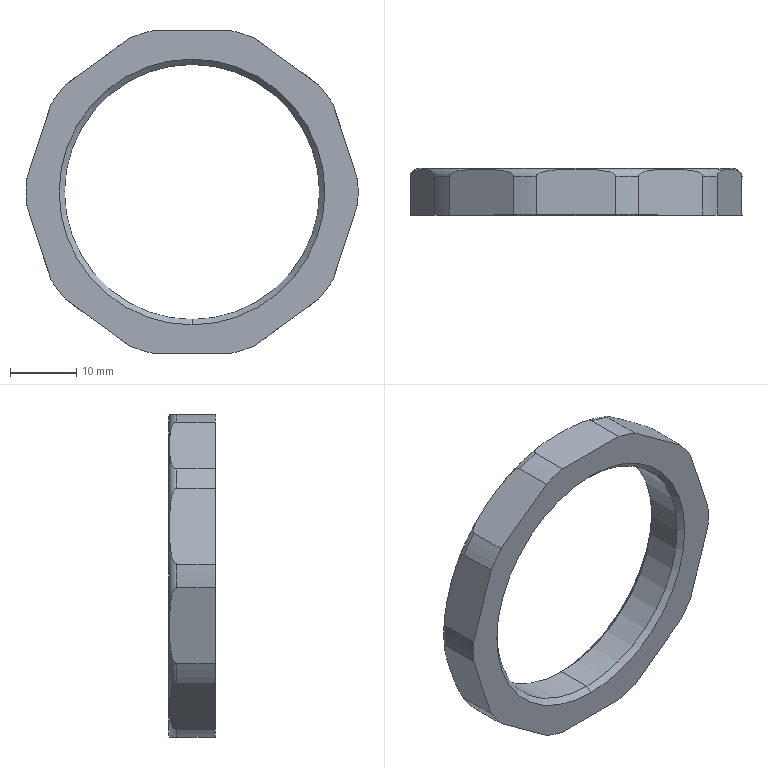Part | SolidWorks | features BaseBody 1 | 1 solid | 30 faces | box 50 x 7 x 48.544 mm | volume 5139 mm3 | cylinder 12 | plane 12 | cone 4 | torus 2 | commonest cylinder face diameters 50 x10 38.376 x2
STEP:
#1=CARTESIAN_POINT('',(5.99,38.8,-24.272));
#2=VERTEX_POINT('',#1);
#3=CARTESIAN_POINT('',(0.,39.903,-24.272));
#4=VERTEX_POINT('',#3);
#5=CARTESIAN_POINT('',(5.99,38.8,-24.272));
#6=CARTESIAN_POINT('',(5.99,38.868,-24.272));
#7=CARTESIAN_POINT('',(5.965,38.932,-24.272));
#8=CARTESIAN_POINT('',(5.891,39.043,-24.272));
#9=CARTESIAN_POINT('',(5.843,39.09,-24.272));
#10=CARTESIAN_POINT('',(5.688,39.215,-24.272));
#11=CARTESIAN_POINT('',(5.569,39.278,-24.272));
#12=CARTESIAN_POINT('',(5.208,39.438,-24.272));
#13=CARTESIAN_POINT('',(4.952,39.51,-24.272));
#14=CARTESIAN_POINT('',(4.439,39.627,-24.272));
#15=CARTESIAN_POINT('',(4.181,39.67,-24.272));
#16=CARTESIAN_POINT('',(3.663,39.742,-24.272));
#17=CARTESIAN_POINT('',(3.403,39.77,-24.272));
#18=CARTESIAN_POINT('',(2.621,39.838,-24.272));
#19=CARTESIAN_POINT('',(2.098,39.864,-24.272));
#20=CARTESIAN_POINT('',(1.049,39.897,-24.272));
#21=CARTESIAN_POINT('',(0.5246,39.903,-24.272));
#22=CARTESIAN_POINT('',(0.,39.903,-24.272));
#23=B_SPLINE_CURVE_WITH_KNOTS('',3,(#5,#6,#7,#8,#9,#10,#11,#12,#13,#14,#15,#16,#17,#18,#19,#20,#21,#22),.UNSPECIFIED.,.F.,.F.,(4,2,2,2,2,2,2,2,4),(-0.006293,-0.006096,-0.0059,-0.005506,-0.00472,-0.003933,-0.003146,-0.001573,0.),.UNSPECIFIED.);
#24=EDGE_CURVE('',#2,#4,#23,.T.);
#25=ORIENTED_EDGE('',*,*,#24,.T.);
#26=CARTESIAN_POINT('',(0.,40.,-23.8));
#27=VERTEX_POINT('',#26);
#28=CARTESIAN_POINT('',(0.,38.8,-23.8));
#29=DIRECTION('',(1.,0.,0.));
#30=DIRECTION('',(0.,0.,-1.));
#31=AXIS2_PLACEMENT_3D('',#28,#29,#30);
#32=CIRCLE('',#31,1.2);
#33=EDGE_CURVE('',#4,#27,#32,.T.);
#34=ORIENTED_EDGE('',*,*,#33,.T.);
#35=CARTESIAN_POINT('',(0.,40.,23.8));
#36=VERTEX_POINT('',#35);
#37=CARTESIAN_POINT('',(0.,40.,0.));
#38=DIRECTION('',(0.,-1.,0.));
#39=DIRECTION('',(0.,0.,1.));
#40=AXIS2_PLACEMENT_3D('',#37,#38,#39);
#41=CIRCLE('',#40,23.8);
#42=EDGE_CURVE('',#27,#36,#41,.T.);
#43=ORIENTED_EDGE('',*,*,#42,.T.);
#44=CARTESIAN_POINT('',(0.,39.903,24.272));
#45=VERTEX_POINT('',#44);
#46=CARTESIAN_POINT('',(0.,38.8,23.8));
#47=DIRECTION('',(-1.,0.,0.));
#48=DIRECTION('',(0.,0.,1.));
#49=AXIS2_PLACEMENT_3D('',#46,#47,#48);
#50=CIRCLE('',#49,1.2);
#51=EDGE_CURVE('',#45,#36,#50,.T.);
#52=ORIENTED_EDGE('',*,*,#51,.F.);
#53=CARTESIAN_POINT('',(5.99,38.8,24.272));
#54=VERTEX_POINT('',#53);
#55=CARTESIAN_POINT('',(0.,39.903,24.272));
#56=CARTESIAN_POINT('',(0.5253,39.903,24.272));
#57=CARTESIAN_POINT('',(1.05,39.897,24.272));
#58=CARTESIAN_POINT('',(2.1,39.864,24.272));
#59=CARTESIAN_POINT('',(2.625,39.838,24.272));
#60=CARTESIAN_POINT('',(3.672,39.746,24.272));
#61=CARTESIAN_POINT('',(4.195,39.683,24.272));
#62=CARTESIAN_POINT('',(4.963,39.507,24.272));
#63=CARTESIAN_POINT('',(5.218,39.435,24.272));
#64=CARTESIAN_POINT('',(5.577,39.274,24.272));
#65=CARTESIAN_POINT('',(5.693,39.212,24.272));
#66=CARTESIAN_POINT('',(5.846,39.087,24.272));
#67=CARTESIAN_POINT('',(5.894,39.04,24.272));
#68=CARTESIAN_POINT('',(5.965,38.931,24.272));
#69=CARTESIAN_POINT('',(5.99,38.867,24.272));
#70=CARTESIAN_POINT('',(5.99,38.8,24.272));
#71=B_SPLINE_CURVE_WITH_KNOTS('',3,(#55,#56,#57,#58,#59,#60,#61,#62,#63,#64,#65,#66,#67,#68,#69,#70),.UNSPECIFIED.,.F.,.F.,(4,2,2,2,2,2,2,4),(0.006368,0.007963,0.009557,0.01115,0.01195,0.01235,0.01255,0.01275),.UNSPECIFIED.);
#72=EDGE_CURVE('',#45,#54,#71,.T.);
#73=ORIENTED_EDGE('',*,*,#72,.T.);
#74=CARTESIAN_POINT('',(9.421,38.8,23.157));
#75=VERTEX_POINT('',#74);
#76=CARTESIAN_POINT('',(0.,38.8,0.));
#77=DIRECTION('',(0.,-1.,0.));
#78=DIRECTION('',(0.,0.,-1.));
#79=AXIS2_PLACEMENT_3D('',#76,#77,#78);
#80=CIRCLE('',#79,25.);
#81=EDGE_CURVE('',#75,#54,#80,.T.);
#82=ORIENTED_EDGE('',*,*,#81,.F.);
#83=CARTESIAN_POINT('',(19.112,38.8,16.116));
#84=VERTEX_POINT('',#83);
#85=CARTESIAN_POINT('',(9.421,38.8,23.157));
#86=CARTESIAN_POINT('',(9.421,38.868,23.157));
#87=CARTESIAN_POINT('',(9.441,38.932,23.142));
#88=CARTESIAN_POINT('',(9.501,39.043,23.099));
#89=CARTESIAN_POINT('',(9.54,39.091,23.071));
#90=CARTESIAN_POINT('',(9.665,39.215,22.979));
#91=CARTESIAN_POINT('',(9.762,39.278,22.909));
#92=CARTESIAN_POINT('',(10.054,39.438,22.697));
#93=CARTESIAN_POINT('',(10.261,39.51,22.546));
#94=CARTESIAN_POINT('',(10.676,39.627,22.245));
#95=CARTESIAN_POINT('',(10.885,39.671,22.093));
#96=CARTESIAN_POINT('',(11.305,39.742,21.788));
#97=CARTESIAN_POINT('',(11.515,39.77,21.635));
#98=CARTESIAN_POINT('',(12.148,39.838,21.175));
#99=CARTESIAN_POINT('',(12.572,39.864,20.867));
#100=CARTESIAN_POINT('',(13.421,39.897,20.251));
#101=CARTESIAN_POINT('',(13.846,39.903,19.942));
#102=CARTESIAN_POINT('',(14.695,39.903,19.325));
#103=CARTESIAN_POINT('',(15.12,39.896,19.017));
#104=CARTESIAN_POINT('',(15.968,39.863,18.4));
#105=CARTESIAN_POINT('',(16.393,39.838,18.092));
#106=CARTESIAN_POINT('',(17.239,39.746,17.477));
#107=CARTESIAN_POINT('',(17.662,39.683,17.17));
#108=CARTESIAN_POINT('',(18.282,39.507,16.719));
#109=CARTESIAN_POINT('',(18.488,39.435,16.569));
#110=CARTESIAN_POINT('',(18.779,39.274,16.358));
#111=CARTESIAN_POINT('',(18.873,39.212,16.29));
#112=CARTESIAN_POINT('',(18.997,39.087,16.2));
#113=CARTESIAN_POINT('',(19.035,39.04,16.172));
#114=CARTESIAN_POINT('',(19.093,38.931,16.13));
#115=CARTESIAN_POINT('',(19.112,38.867,16.116));
#116=CARTESIAN_POINT('',(19.112,38.8,16.116));
#117=B_SPLINE_CURVE_WITH_KNOTS('',3,(#85,#86,#87,#88,#89,#90,#91,#92,#93,#94,#95,#96,#97,#98,#99,#100,#101,#102,#103,#104,#105,#106,#107,#108,#109,#110,#111,#112,#113,#114,#115,#116),.UNSPECIFIED.,.F.,.F.,(4,2,2,2,2,2,2,2,2,2,2,2,2,2,2,4),(0.,0.0001992,0.0003983,0.0007966,0.001593,0.00239,0.003187,0.00478,0.006373,0.007966,0.00956,0.01115,0.01195,0.01235,0.01255,0.01275),.UNSPECIFIED.);
#118=EDGE_CURVE('',#75,#84,#117,.T.);
#119=ORIENTED_EDGE('',*,*,#118,.T.);
#120=CARTESIAN_POINT('',(21.233,38.8,13.197));
#121=VERTEX_POINT('',#120);
#122=CARTESIAN_POINT('',(0.,38.8,0.));
#123=DIRECTION('',(0.,-1.,0.));
#124=DIRECTION('',(0.,0.,-1.));
#125=AXIS2_PLACEMENT_3D('',#122,#123,#124);
#126=CIRCLE('',#125,25.);
#127=EDGE_CURVE('',#121,#84,#126,.T.);
#128=ORIENTED_EDGE('',*,*,#127,.F.);
#129=CARTESIAN_POINT('',(24.935,38.8,1.804));
#130=VERTEX_POINT('',#129);
#131=CARTESIAN_POINT('',(21.233,38.8,13.197));
#132=CARTESIAN_POINT('',(21.233,38.868,13.197));
#133=CARTESIAN_POINT('',(21.241,38.932,13.173));
#134=CARTESIAN_POINT('',(21.263,39.043,13.103));
#135=CARTESIAN_POINT('',(21.278,39.091,13.057));
#136=CARTESIAN_POINT('',(21.326,39.215,12.91));
#137=CARTESIAN_POINT('',(21.363,39.278,12.796));
#138=CARTESIAN_POINT('',(21.475,39.438,12.453));
#139=CARTESIAN_POINT('',(21.554,39.51,12.209));
#140=CARTESIAN_POINT('',(21.713,39.627,11.721));
#141=CARTESIAN_POINT('',(21.792,39.671,11.475));
#142=CARTESIAN_POINT('',(21.953,39.742,10.982));
#143=CARTESIAN_POINT('',(22.033,39.77,10.735));
#144=CARTESIAN_POINT('',(22.275,39.838,9.991));
#145=CARTESIAN_POINT('',(22.437,39.864,9.492));
#146=CARTESIAN_POINT('',(22.761,39.897,8.494));
#147=CARTESIAN_POINT('',(22.923,39.903,7.995));
#148=CARTESIAN_POINT('',(23.247,39.903,6.997));
#149=CARTESIAN_POINT('',(23.41,39.896,6.498));
#150=CARTESIAN_POINT('',(23.734,39.863,5.5));
#151=CARTESIAN_POINT('',(23.896,39.838,5.001));
#152=CARTESIAN_POINT('',(24.219,39.746,4.007));
#153=CARTESIAN_POINT('',(24.381,39.683,3.509));
#154=CARTESIAN_POINT('',(24.618,39.507,2.78));
#155=CARTESIAN_POINT('',(24.696,39.435,2.537));
#156=CARTESIAN_POINT('',(24.807,39.274,2.196));
#157=CARTESIAN_POINT('',(24.843,39.212,2.085));
#158=CARTESIAN_POINT('',(24.891,39.087,1.94));
#159=CARTESIAN_POINT('',(24.905,39.04,1.895));
#160=CARTESIAN_POINT('',(24.927,38.931,1.827));
#161=CARTESIAN_POINT('',(24.935,38.867,1.804));
#162=CARTESIAN_POINT('',(24.935,38.8,1.804));
#163=B_SPLINE_CURVE_WITH_KNOTS('',3,(#131,#132,#133,#134,#135,#136,#137,#138,#139,#140,#141,#142,#143,#144,#145,#146,#147,#148,#149,#150,#151,#152,#153,#154,#155,#156,#157,#158,#159,#160,#161,#162),.UNSPECIFIED.,.F.,.F.,(4,2,2,2,2,2,2,2,2,2,2,2,2,2,2,4),(0.,0.0001992,0.0003983,0.0007966,0.001593,0.00239,0.003187,0.00478,0.006373,0.007966,0.00956,0.01115,0.01195,0.01235,0.01255,0.01275),.UNSPECIFIED.);
#164=EDGE_CURVE('',#121,#130,#163,.T.);
#165=ORIENTED_EDGE('',*,*,#164,.T.);
#166=CARTESIAN_POINT('',(24.935,38.8,-1.804));
#167=VERTEX_POINT('',#166);
#168=CARTESIAN_POINT('',(0.,38.8,0.));
#169=DIRECTION('',(0.,-1.,0.));
#170=DIRECTION('',(0.,0.,-1.));
#171=AXIS2_PLACEMENT_3D('',#168,#169,#170);
#172=CIRCLE('',#171,25.);
#173=EDGE_CURVE('',#167,#130,#172,.T.);
#174=ORIENTED_EDGE('',*,*,#173,.F.);
#175=CARTESIAN_POINT('',(21.233,38.8,-13.197));
#176=VERTEX_POINT('',#175);
#177=CARTESIAN_POINT('',(24.935,38.8,-1.804));
#178=CARTESIAN_POINT('',(24.935,38.868,-1.804));
#179=CARTESIAN_POINT('',(24.927,38.932,-1.827));
#180=CARTESIAN_POINT('',(24.904,39.043,-1.898));
#181=CARTESIAN_POINT('',(24.889,39.091,-1.944));
#182=CARTESIAN_POINT('',(24.841,39.215,-2.091));
#183=CARTESIAN_POINT('',(24.805,39.278,-2.204));
#184=CARTESIAN_POINT('',(24.693,39.438,-2.548));
#185=CARTESIAN_POINT('',(24.614,39.51,-2.792));
#186=CARTESIAN_POINT('',(24.455,39.627,-3.28));
#187=CARTESIAN_POINT('',(24.375,39.671,-3.525));
#188=CARTESIAN_POINT('',(24.215,39.742,-4.019));
#189=CARTESIAN_POINT('',(24.135,39.77,-4.266));
#190=CARTESIAN_POINT('',(23.893,39.838,-5.01));
#191=CARTESIAN_POINT('',(23.731,39.864,-5.509));
#192=CARTESIAN_POINT('',(23.407,39.897,-6.506));
#193=CARTESIAN_POINT('',(23.245,39.903,-7.006));
#194=CARTESIAN_POINT('',(22.92,39.903,-8.004));
#195=CARTESIAN_POINT('',(22.758,39.896,-8.503));
#196=CARTESIAN_POINT('',(22.434,39.863,-9.501));
#197=CARTESIAN_POINT('',(22.272,39.838,-10.));
#198=CARTESIAN_POINT('',(21.949,39.746,-10.994));
#199=CARTESIAN_POINT('',(21.787,39.683,-11.492));
#200=CARTESIAN_POINT('',(21.55,39.507,-12.221));
#201=CARTESIAN_POINT('',(21.471,39.435,-12.463));
#202=CARTESIAN_POINT('',(21.36,39.274,-12.805));
#203=CARTESIAN_POINT('',(21.324,39.212,-12.915));
#204=CARTESIAN_POINT('',(21.277,39.087,-13.061));
#205=CARTESIAN_POINT('',(21.263,39.04,-13.106));
#206=CARTESIAN_POINT('',(21.24,38.931,-13.174));
#207=CARTESIAN_POINT('',(21.233,38.867,-13.197));
#208=CARTESIAN_POINT('',(21.233,38.8,-13.197));
#209=B_SPLINE_CURVE_WITH_KNOTS('',3,(#177,#178,#179,#180,#181,#182,#183,#184,#185,#186,#187,#188,#189,#190,#191,#192,#193,#194,#195,#196,#197,#198,#199,#200,#201,#202,#203,#204,#205,#206,#207,#208),.UNSPECIFIED.,.F.,.F.,(4,2,2,2,2,2,2,2,2,2,2,2,2,2,2,4),(0.,0.0001992,0.0003983,0.0007966,0.001593,0.00239,0.003187,0.00478,0.006373,0.007966,0.00956,0.01115,0.01195,0.01235,0.01255,0.01275),.UNSPECIFIED.);
#210=EDGE_CURVE('',#167,#176,#209,.T.);
#211=ORIENTED_EDGE('',*,*,#210,.T.);
#212=CARTESIAN_POINT('',(19.112,38.8,-16.116));
#213=VERTEX_POINT('',#212);
#214=CARTESIAN_POINT('',(0.,38.8,0.));
#215=DIRECTION('',(0.,-1.,0.));
#216=DIRECTION('',(0.,0.,-1.));
#217=AXIS2_PLACEMENT_3D('',#214,#215,#216);
#218=CIRCLE('',#217,25.);
#219=EDGE_CURVE('',#213,#176,#218,.T.);
#220=ORIENTED_EDGE('',*,*,#219,.F.);
#221=CARTESIAN_POINT('',(9.421,38.8,-23.157));
#222=VERTEX_POINT('',#221);
#223=CARTESIAN_POINT('',(19.112,38.8,-16.116));
#224=CARTESIAN_POINT('',(19.112,38.868,-16.116));
#225=CARTESIAN_POINT('',(19.092,38.932,-16.13));
#226=CARTESIAN_POINT('',(19.033,39.043,-16.174));
#227=CARTESIAN_POINT('',(18.993,39.091,-16.202));
#228=CARTESIAN_POINT('',(18.868,39.215,-16.293));
#229=CARTESIAN_POINT('',(18.772,39.278,-16.363));
#230=CARTESIAN_POINT('',(18.48,39.438,-16.575));
#231=CARTESIAN_POINT('',(18.272,39.51,-16.726));
#232=CARTESIAN_POINT('',(17.857,39.627,-17.028));
#233=CARTESIAN_POINT('',(17.648,39.671,-17.18));
#234=CARTESIAN_POINT('',(17.228,39.742,-17.484));
#235=CARTESIAN_POINT('',(17.018,39.77,-17.637));
#236=CARTESIAN_POINT('',(16.385,39.838,-18.097));
#237=CARTESIAN_POINT('',(15.961,39.864,-18.405));
#238=CARTESIAN_POINT('',(15.112,39.897,-19.022));
#239=CARTESIAN_POINT('',(14.688,39.903,-19.33));
#240=CARTESIAN_POINT('',(13.838,39.903,-19.947));
#241=CARTESIAN_POINT('',(13.414,39.896,-20.256));
#242=CARTESIAN_POINT('',(12.565,39.863,-20.873));
#243=CARTESIAN_POINT('',(12.14,39.838,-21.181));
#244=CARTESIAN_POINT('',(11.295,39.746,-21.796));
#245=CARTESIAN_POINT('',(10.872,39.683,-22.103));
#246=CARTESIAN_POINT('',(10.251,39.507,-22.554));
#247=CARTESIAN_POINT('',(10.045,39.435,-22.704));
#248=CARTESIAN_POINT('',(9.755,39.274,-22.914));
#249=CARTESIAN_POINT('',(9.66,39.212,-22.983));
#250=CARTESIAN_POINT('',(9.537,39.087,-23.073));
#251=CARTESIAN_POINT('',(9.498,39.04,-23.101));
#252=CARTESIAN_POINT('',(9.44,38.931,-23.143));
#253=CARTESIAN_POINT('',(9.421,38.867,-23.157));
#254=CARTESIAN_POINT('',(9.421,38.8,-23.157));
#255=B_SPLINE_CURVE_WITH_KNOTS('',3,(#223,#224,#225,#226,#227,#228,#229,#230,#231,#232,#233,#234,#235,#236,#237,#238,#239,#240,#241,#242,#243,#244,#245,#246,#247,#248,#249,#250,#251,#252,#253,#254),.UNSPECIFIED.,.F.,.F.,(4,2,2,2,2,2,2,2,2,2,2,2,2,2,2,4),(0.,0.0001992,0.0003983,0.0007966,0.001593,0.00239,0.003187,0.00478,0.006373,0.007966,0.00956,0.01115,0.01195,0.01235,0.01255,0.01275),.UNSPECIFIED.);
#256=EDGE_CURVE('',#213,#222,#255,.T.);
#257=ORIENTED_EDGE('',*,*,#256,.T.);
#258=CARTESIAN_POINT('',(0.,38.8,0.));
#259=DIRECTION('',(0.,-1.,0.));
#260=DIRECTION('',(0.,0.,-1.));
#261=AXIS2_PLACEMENT_3D('',#258,#259,#260);
#262=CIRCLE('',#261,25.);
#263=EDGE_CURVE('',#2,#222,#262,.T.);
#264=ORIENTED_EDGE('',*,*,#263,.F.);
#265=EDGE_LOOP('',(#25,#34,#43,#52,#73,#82,#119,#128,#165,#174,#211,#220,#257,#264));
#266=FACE_OUTER_BOUND('',#265,.T.);
#267=CARTESIAN_POINT('',(0.,38.8,0.));
#268=DIRECTION('',(0.,1.,0.));
#269=DIRECTION('',(0.,0.,1.));
#270=AXIS2_PLACEMENT_3D('',#267,#268,#269);
#271=TOROIDAL_SURFACE('',#270,23.8,1.2);
#272=ADVANCED_FACE('',(#266),#271,.T.);
#273=CARTESIAN_POINT('',(0.,33.812,19.188));
#274=VERTEX_POINT('',#273);
#275=CARTESIAN_POINT('',(0.,33.812,-19.188));
#276=VERTEX_POINT('',#275);
#277=CARTESIAN_POINT('',(0.,33.812,0.));
#278=DIRECTION('',(0.,-1.,0.));
#279=DIRECTION('',(1.,0.,0.));
#280=AXIS2_PLACEMENT_3D('',#277,#278,#279);
#281=CIRCLE('',#280,19.188);
#282=EDGE_CURVE('',#274,#276,#281,.T.);
#283=ORIENTED_EDGE('',*,*,#282,.F.);
#284=CARTESIAN_POINT('',(0.,33.,20.));
#285=VERTEX_POINT('',#284);
#286=CARTESIAN_POINT('',(0.,33.,20.));
#287=DIRECTION('',(0.,-0.7071,0.7071));
#288=VECTOR('',#287,1000.);
#289=LINE('',#286,#288);
#290=EDGE_CURVE('',#274,#285,#289,.T.);
#291=ORIENTED_EDGE('',*,*,#290,.T.);
#292=CARTESIAN_POINT('',(0.,33.,-20.));
#293=VERTEX_POINT('',#292);
#294=CARTESIAN_POINT('',(0.,33.,0.));
#295=DIRECTION('',(0.,1.,0.));
#296=DIRECTION('',(0.,0.,-1.));
#297=AXIS2_PLACEMENT_3D('',#294,#295,#296);
#298=CIRCLE('',#297,20.);
#299=EDGE_CURVE('',#293,#285,#298,.T.);
#300=ORIENTED_EDGE('',*,*,#299,.F.);
#301=CARTESIAN_POINT('',(0.,33.,-20.));
#302=DIRECTION('',(0.,-0.7071,-0.7071));
#303=VECTOR('',#302,1000.);
#304=LINE('',#301,#303);
#305=EDGE_CURVE('',#276,#293,#304,.T.);
#306=ORIENTED_EDGE('',*,*,#305,.F.);
#307=EDGE_LOOP('',(#283,#291,#300,#306));
#308=FACE_OUTER_BOUND('',#307,.T.);
#309=CARTESIAN_POINT('',(0.,33.,0.));
#310=DIRECTION('',(0.,-1.,0.));
#311=DIRECTION('',(0.,0.,-1.));
#312=AXIS2_PLACEMENT_3D('',#309,#310,#311);
#313=CONICAL_SURFACE('',#312,20.,0.7854);
#314=ADVANCED_FACE('',(#308),#313,.F.);
#315=CARTESIAN_POINT('',(0.,39.188,19.188));
#316=VERTEX_POINT('',#315);
#317=CARTESIAN_POINT('',(0.,39.188,-19.188));
#318=VERTEX_POINT('',#317);
#319=CARTESIAN_POINT('',(0.,39.188,0.));
#320=DIRECTION('',(0.,-1.,0.));
#321=DIRECTION('',(0.,0.,-1.));
#322=AXIS2_PLACEMENT_3D('',#319,#320,#321);
#323=CIRCLE('',#322,19.188);
#324=EDGE_CURVE('',#316,#318,#323,.T.);
#325=ORIENTED_EDGE('',*,*,#324,.F.);
#326=CARTESIAN_POINT('',(0.,36.5,19.188));
#327=DIRECTION('',(0.,-1.,0.));
#328=VECTOR('',#327,1000.);
#329=LINE('',#326,#328);
#330=EDGE_CURVE('',#316,#274,#329,.T.);
#331=ORIENTED_EDGE('',*,*,#330,.T.);
#332=ORIENTED_EDGE('',*,*,#282,.T.);
#333=CARTESIAN_POINT('',(0.,36.5,-19.188));
#334=DIRECTION('',(0.,-1.,0.));
#335=VECTOR('',#334,1000.);
#336=LINE('',#333,#335);
#337=EDGE_CURVE('',#318,#276,#336,.T.);
#338=ORIENTED_EDGE('',*,*,#337,.F.);
#339=EDGE_LOOP('',(#325,#331,#332,#338));
#340=FACE_OUTER_BOUND('',#339,.T.);
#341=CARTESIAN_POINT('',(0.,36.5,0.));
#342=DIRECTION('',(0.,-1.,0.));
#343=DIRECTION('',(0.,0.,-1.));
#344=AXIS2_PLACEMENT_3D('',#341,#342,#343);
#345=CYLINDRICAL_SURFACE('',#344,19.188);
#346=ADVANCED_FACE('',(#340),#345,.F.);
#347=ORIENTED_EDGE('',*,*,#324,.T.);
#348=CARTESIAN_POINT('',(0.,40.,-20.));
#349=VERTEX_POINT('',#348);
#350=CARTESIAN_POINT('',(0.,40.,-20.));
#351=DIRECTION('',(0.,0.7071,-0.7071));
#352=VECTOR('',#351,1000.);
#353=LINE('',#350,#352);
#354=EDGE_CURVE('',#318,#349,#353,.T.);
#355=ORIENTED_EDGE('',*,*,#354,.T.);
#356=CARTESIAN_POINT('',(0.,40.,20.));
#357=VERTEX_POINT('',#356);
#358=CARTESIAN_POINT('',(0.,40.,0.));
#359=DIRECTION('',(0.,-1.,0.));
#360=DIRECTION('',(0.,0.,1.));
#361=AXIS2_PLACEMENT_3D('',#358,#359,#360);
#362=CIRCLE('',#361,20.);
#363=EDGE_CURVE('',#357,#349,#362,.T.);
#364=ORIENTED_EDGE('',*,*,#363,.F.);
#365=CARTESIAN_POINT('',(0.,40.,20.));
#366=DIRECTION('',(0.,0.7071,0.7071));
#367=VECTOR('',#366,1000.);
#368=LINE('',#365,#367);
#369=EDGE_CURVE('',#316,#357,#368,.T.);
#370=ORIENTED_EDGE('',*,*,#369,.F.);
#371=EDGE_LOOP('',(#347,#355,#364,#370));
#372=FACE_OUTER_BOUND('',#371,.T.);
#373=CARTESIAN_POINT('',(0.,40.,0.));
#374=DIRECTION('',(0.,1.,0.));
#375=DIRECTION('',(0.,0.,1.));
#376=AXIS2_PLACEMENT_3D('',#373,#374,#375);
#377=CONICAL_SURFACE('',#376,20.,0.7854);
#378=ADVANCED_FACE('',(#372),#377,.F.);
#379=ORIENTED_EDGE('',*,*,#363,.T.);
#380=CARTESIAN_POINT('',(0.,40.,0.));
#381=DIRECTION('',(0.,-1.,0.));
#382=DIRECTION('',(0.,0.,1.));
#383=AXIS2_PLACEMENT_3D('',#380,#381,#382);
#384=CIRCLE('',#383,20.);
#385=EDGE_CURVE('',#349,#357,#384,.T.);
#386=ORIENTED_EDGE('',*,*,#385,.T.);
#387=EDGE_LOOP('',(#379,#386));
#388=FACE_BOUND('',#387,.T.);
#389=CARTESIAN_POINT('',(0.,40.,0.));
#390=DIRECTION('',(0.,-1.,0.));
#391=DIRECTION('',(0.,0.,1.));
#392=AXIS2_PLACEMENT_3D('',#389,#390,#391);
#393=CIRCLE('',#392,23.8);
#394=EDGE_CURVE('',#36,#27,#393,.T.);
#395=ORIENTED_EDGE('',*,*,#394,.F.);
#396=ORIENTED_EDGE('',*,*,#42,.F.);
#397=EDGE_LOOP('',(#395,#396));
#398=FACE_OUTER_BOUND('',#397,.T.);
#399=CARTESIAN_POINT('',(21.9,40.,0.));
#400=DIRECTION('',(0.,1.,0.));
#401=DIRECTION('',(1.,0.,0.));
#402=AXIS2_PLACEMENT_3D('',#399,#400,#401);
#403=PLANE('',#402);
#404=ADVANCED_FACE('',(#388,#398),#403,.T.);
#405=CARTESIAN_POINT('',(-19.112,33.,-16.116));
#406=VERTEX_POINT('',#405);
#407=CARTESIAN_POINT('',(-9.421,33.,-23.157));
#408=VERTEX_POINT('',#407);
#409=CARTESIAN_POINT('',(-19.112,33.,-16.116));
#410=DIRECTION('',(0.809,0.,-0.5878));
#411=VECTOR('',#410,1000.);
#412=LINE('',#409,#411);
#413=EDGE_CURVE('',#406,#408,#412,.T.);
#414=ORIENTED_EDGE('',*,*,#413,.F.);
#415=CARTESIAN_POINT('',(-19.112,38.8,-16.116));
#416=VERTEX_POINT('',#415);
#417=CARTESIAN_POINT('',(-19.112,35.9,-16.116));
#418=DIRECTION('',(0.,-1.,0.));
#419=VECTOR('',#418,1000.);
#420=LINE('',#417,#419);
#421=EDGE_CURVE('',#416,#406,#420,.T.);
#422=ORIENTED_EDGE('',*,*,#421,.F.);
#423=CARTESIAN_POINT('',(-9.421,38.8,-23.157));
#424=VERTEX_POINT('',#423);
#425=CARTESIAN_POINT('',(-9.421,38.8,-23.157));
#426=CARTESIAN_POINT('',(-9.421,38.868,-23.157));
#427=CARTESIAN_POINT('',(-9.441,38.932,-23.142));
#428=CARTESIAN_POINT('',(-9.501,39.043,-23.099));
#429=CARTESIAN_POINT('',(-9.54,39.091,-23.071));
#430=CARTESIAN_POINT('',(-9.665,39.215,-22.979));
#431=CARTESIAN_POINT('',(-9.762,39.278,-22.909));
#432=CARTESIAN_POINT('',(-10.054,39.438,-22.697));
#433=CARTESIAN_POINT('',(-10.261,39.51,-22.546));
#434=CARTESIAN_POINT('',(-10.676,39.627,-22.245));
#435=CARTESIAN_POINT('',(-10.885,39.671,-22.093));
#436=CARTESIAN_POINT('',(-11.305,39.742,-21.788));
#437=CARTESIAN_POINT('',(-11.515,39.77,-21.635));
#438=CARTESIAN_POINT('',(-12.148,39.838,-21.175));
#439=CARTESIAN_POINT('',(-12.572,39.864,-20.867));
#440=CARTESIAN_POINT('',(-13.421,39.897,-20.251));
#441=CARTESIAN_POINT('',(-13.846,39.903,-19.942));
#442=CARTESIAN_POINT('',(-14.695,39.903,-19.325));
#443=CARTESIAN_POINT('',(-15.12,39.896,-19.017));
#444=CARTESIAN_POINT('',(-15.968,39.863,-18.4));
#445=CARTESIAN_POINT('',(-16.393,39.838,-18.092));
#446=CARTESIAN_POINT('',(-17.239,39.746,-17.477));
#447=CARTESIAN_POINT('',(-17.662,39.683,-17.17));
#448=CARTESIAN_POINT('',(-18.282,39.507,-16.719));
#449=CARTESIAN_POINT('',(-18.488,39.435,-16.569));
#450=CARTESIAN_POINT('',(-18.779,39.274,-16.358));
#451=CARTESIAN_POINT('',(-18.873,39.212,-16.29));
#452=CARTESIAN_POINT('',(-18.997,39.087,-16.2));
#453=CARTESIAN_POINT('',(-19.035,39.04,-16.172));
#454=CARTESIAN_POINT('',(-19.093,38.931,-16.13));
#455=CARTESIAN_POINT('',(-19.112,38.867,-16.116));
#456=CARTESIAN_POINT('',(-19.112,38.8,-16.116));
#457=B_SPLINE_CURVE_WITH_KNOTS('',3,(#425,#426,#427,#428,#429,#430,#431,#432,#433,#434,#435,#436,#437,#438,#439,#440,#441,#442,#443,#444,#445,#446,#447,#448,#449,#450,#451,#452,#453,#454,#455,#456),.UNSPECIFIED.,.F.,.F.,(4,2,2,2,2,2,2,2,2,2,2,2,2,2,2,4),(0.,0.0001992,0.0003983,0.0007966,0.001593,0.00239,0.003187,0.00478,0.006373,0.007966,0.00956,0.01115,0.01195,0.01235,0.01255,0.01275),.UNSPECIFIED.);
#458=EDGE_CURVE('',#424,#416,#457,.T.);
#459=ORIENTED_EDGE('',*,*,#458,.F.);
#460=CARTESIAN_POINT('',(-9.421,35.9,-23.157));
#461=DIRECTION('',(0.,1.,0.));
#462=VECTOR('',#461,1000.);
#463=LINE('',#460,#462);
#464=EDGE_CURVE('',#408,#424,#463,.T.);
#465=ORIENTED_EDGE('',*,*,#464,.F.);
#466=EDGE_LOOP('',(#414,#422,#459,#465));
#467=FACE_OUTER_BOUND('',#466,.T.);
#468=CARTESIAN_POINT('',(-19.44,40.,-15.878));
#469=DIRECTION('',(0.5878,0.,0.809));
#470=DIRECTION('',(0.,-1.,0.));
#471=AXIS2_PLACEMENT_3D('',#468,#469,#470);
#472=PLANE('',#471);
#473=ADVANCED_FACE('',(#467),#472,.F.);
#474=CARTESIAN_POINT('',(-5.99,38.8,-24.272));
#475=VERTEX_POINT('',#474);
#476=CARTESIAN_POINT('',(-5.99,33.,-24.272));
#477=VERTEX_POINT('',#476);
#478=CARTESIAN_POINT('',(-5.99,40.,-24.272));
#479=DIRECTION('',(0.,-1.,0.));
#480=VECTOR('',#479,1000.);
#481=LINE('',#478,#480);
#482=EDGE_CURVE('',#475,#477,#481,.T.);
#483=ORIENTED_EDGE('',*,*,#482,.T.);
#484=CARTESIAN_POINT('',(0.,33.,0.));
#485=DIRECTION('',(0.,-1.,0.));
#486=DIRECTION('',(0.,0.,-1.));
#487=AXIS2_PLACEMENT_3D('',#484,#485,#486);
#488=CIRCLE('',#487,25.);
#489=EDGE_CURVE('',#408,#477,#488,.T.);
#490=ORIENTED_EDGE('',*,*,#489,.F.);
#491=ORIENTED_EDGE('',*,*,#464,.T.);
#492=CARTESIAN_POINT('',(0.,38.8,0.));
#493=DIRECTION('',(0.,-1.,0.));
#494=DIRECTION('',(0.,0.,-1.));
#495=AXIS2_PLACEMENT_3D('',#492,#493,#494);
#496=CIRCLE('',#495,25.);
#497=EDGE_CURVE('',#424,#475,#496,.T.);
#498=ORIENTED_EDGE('',*,*,#497,.T.);
#499=EDGE_LOOP('',(#483,#490,#491,#498));
#500=FACE_OUTER_BOUND('',#499,.T.);
#501=CARTESIAN_POINT('',(0.,35.9,0.));
#502=DIRECTION('',(0.,-1.,0.));
#503=DIRECTION('',(0.,0.,-1.));
#504=AXIS2_PLACEMENT_3D('',#501,#502,#503);
#505=CYLINDRICAL_SURFACE('',#504,25.);
#506=ADVANCED_FACE('',(#500),#505,.T.);
#507=CARTESIAN_POINT('',(5.99,33.,-24.272));
#508=VERTEX_POINT('',#507);
#509=CARTESIAN_POINT('',(22.5,33.,-24.272));
#510=DIRECTION('',(1.,0.,0.));
#511=VECTOR('',#510,1000.);
#512=LINE('',#509,#511);
#513=EDGE_CURVE('',#477,#508,#512,.T.);
#514=ORIENTED_EDGE('',*,*,#513,.F.);
#515=ORIENTED_EDGE('',*,*,#482,.F.);
#516=CARTESIAN_POINT('',(0.,39.903,-24.272));
#517=CARTESIAN_POINT('',(-0.5253,39.903,-24.272));
#518=CARTESIAN_POINT('',(-1.05,39.897,-24.272));
#519=CARTESIAN_POINT('',(-2.1,39.864,-24.272));
#520=CARTESIAN_POINT('',(-2.625,39.838,-24.272));
#521=CARTESIAN_POINT('',(-3.672,39.746,-24.272));
#522=CARTESIAN_POINT('',(-4.195,39.683,-24.272));
#523=CARTESIAN_POINT('',(-4.963,39.507,-24.272));
#524=CARTESIAN_POINT('',(-5.218,39.435,-24.272));
#525=CARTESIAN_POINT('',(-5.577,39.274,-24.272));
#526=CARTESIAN_POINT('',(-5.693,39.212,-24.272));
#527=CARTESIAN_POINT('',(-5.846,39.087,-24.272));
#528=CARTESIAN_POINT('',(-5.894,39.04,-24.272));
#529=CARTESIAN_POINT('',(-5.965,38.931,-24.272));
#530=CARTESIAN_POINT('',(-5.99,38.867,-24.272));
#531=CARTESIAN_POINT('',(-5.99,38.8,-24.272));
#532=B_SPLINE_CURVE_WITH_KNOTS('',3,(#516,#517,#518,#519,#520,#521,#522,#523,#524,#525,#526,#527,#528,#529,#530,#531),.UNSPECIFIED.,.F.,.F.,(4,2,2,2,2,2,2,4),(0.,0.001575,0.003151,0.004726,0.005514,0.005908,0.006105,0.006302),.UNSPECIFIED.);
#533=EDGE_CURVE('',#4,#475,#532,.T.);
#534=ORIENTED_EDGE('',*,*,#533,.F.);
#535=ORIENTED_EDGE('',*,*,#24,.F.);
#536=CARTESIAN_POINT('',(5.99,35.9,-24.272));
#537=DIRECTION('',(0.,1.,0.));
#538=VECTOR('',#537,1000.);
#539=LINE('',#536,#538);
#540=EDGE_CURVE('',#508,#2,#539,.T.);
#541=ORIENTED_EDGE('',*,*,#540,.F.);
#542=EDGE_LOOP('',(#514,#515,#534,#535,#541));
#543=FACE_OUTER_BOUND('',#542,.T.);
#544=CARTESIAN_POINT('',(-6.394,40.,-24.272));
#545=DIRECTION('',(0.,0.,1.));
#546=DIRECTION('',(1.,0.,0.));
#547=AXIS2_PLACEMENT_3D('',#544,#545,#546);
#548=PLANE('',#547);
#549=ADVANCED_FACE('',(#543),#548,.F.);
#550=CARTESIAN_POINT('',(9.421,33.,-23.157));
#551=VERTEX_POINT('',#550);
#552=CARTESIAN_POINT('',(9.421,40.,-23.157));
#553=DIRECTION('',(0.,-1.,0.));
#554=VECTOR('',#553,1000.);
#555=LINE('',#552,#554);
#556=EDGE_CURVE('',#222,#551,#555,.T.);
#557=ORIENTED_EDGE('',*,*,#556,.T.);
#558=CARTESIAN_POINT('',(0.,33.,0.));
#559=DIRECTION('',(0.,-1.,0.));
#560=DIRECTION('',(0.,0.,-1.));
#561=AXIS2_PLACEMENT_3D('',#558,#559,#560);
#562=CIRCLE('',#561,25.);
#563=EDGE_CURVE('',#508,#551,#562,.T.);
#564=ORIENTED_EDGE('',*,*,#563,.F.);
#565=ORIENTED_EDGE('',*,*,#540,.T.);
#566=ORIENTED_EDGE('',*,*,#263,.T.);
#567=EDGE_LOOP('',(#557,#564,#565,#566));
#568=FACE_OUTER_BOUND('',#567,.T.);
#569=CARTESIAN_POINT('',(0.,35.9,0.));
#570=DIRECTION('',(0.,-1.,0.));
#571=DIRECTION('',(0.,0.,-1.));
#572=AXIS2_PLACEMENT_3D('',#569,#570,#571);
#573=CYLINDRICAL_SURFACE('',#572,25.);
#574=ADVANCED_FACE('',(#568),#573,.T.);
#575=CARTESIAN_POINT('',(19.112,33.,-16.116));
#576=VERTEX_POINT('',#575);
#577=CARTESIAN_POINT('',(9.421,33.,-23.157));
#578=DIRECTION('',(0.809,0.,0.5878));
#579=VECTOR('',#578,1000.);
#580=LINE('',#577,#579);
#581=EDGE_CURVE('',#551,#576,#580,.T.);
#582=ORIENTED_EDGE('',*,*,#581,.F.);
#583=ORIENTED_EDGE('',*,*,#556,.F.);
#584=ORIENTED_EDGE('',*,*,#256,.F.);
#585=CARTESIAN_POINT('',(19.112,35.9,-16.116));
#586=DIRECTION('',(0.,1.,0.));
#587=VECTOR('',#586,1000.);
#588=LINE('',#585,#587);
#589=EDGE_CURVE('',#576,#213,#588,.T.);
#590=ORIENTED_EDGE('',*,*,#589,.F.);
#591=EDGE_LOOP('',(#582,#583,#584,#590));
#592=FACE_OUTER_BOUND('',#591,.T.);
#593=CARTESIAN_POINT('',(9.094,40.,-23.395));
#594=DIRECTION('',(-0.5878,0.,0.809));
#595=DIRECTION('',(0.,1.,0.));
#596=AXIS2_PLACEMENT_3D('',#593,#594,#595);
#597=PLANE('',#596);
#598=ADVANCED_FACE('',(#592),#597,.F.);
#599=CARTESIAN_POINT('',(21.233,33.,-13.197));
#600=VERTEX_POINT('',#599);
#601=CARTESIAN_POINT('',(21.233,40.,-13.197));
#602=DIRECTION('',(0.,-1.,0.));
#603=VECTOR('',#602,1000.);
#604=LINE('',#601,#603);
#605=EDGE_CURVE('',#176,#600,#604,.T.);
#606=ORIENTED_EDGE('',*,*,#605,.T.);
#607=CARTESIAN_POINT('',(0.,33.,0.));
#608=DIRECTION('',(0.,-1.,0.));
#609=DIRECTION('',(0.,0.,-1.));
#610=AXIS2_PLACEMENT_3D('',#607,#608,#609);
#611=CIRCLE('',#610,25.);
#612=EDGE_CURVE('',#576,#600,#611,.T.);
#613=ORIENTED_EDGE('',*,*,#612,.F.);
#614=ORIENTED_EDGE('',*,*,#589,.T.);
#615=ORIENTED_EDGE('',*,*,#219,.T.);
#616=EDGE_LOOP('',(#606,#613,#614,#615));
#617=FACE_OUTER_BOUND('',#616,.T.);
#618=CARTESIAN_POINT('',(0.,35.9,0.));
#619=DIRECTION('',(0.,-1.,0.));
#620=DIRECTION('',(0.,0.,-1.));
#621=AXIS2_PLACEMENT_3D('',#618,#619,#620);
#622=CYLINDRICAL_SURFACE('',#621,25.);
#623=ADVANCED_FACE('',(#617),#622,.T.);
#624=CARTESIAN_POINT('',(24.935,33.,-1.804));
#625=VERTEX_POINT('',#624);
#626=CARTESIAN_POINT('',(21.233,33.,-13.197));
#627=DIRECTION('',(0.309,0.,0.9511));
#628=VECTOR('',#627,1000.);
#629=LINE('',#626,#628);
#630=EDGE_CURVE('',#600,#625,#629,.T.);
#631=ORIENTED_EDGE('',*,*,#630,.F.);
#632=ORIENTED_EDGE('',*,*,#605,.F.);
#633=ORIENTED_EDGE('',*,*,#210,.F.);
#634=CARTESIAN_POINT('',(24.935,35.9,-1.804));
#635=DIRECTION('',(0.,1.,0.));
#636=VECTOR('',#635,1000.);
#637=LINE('',#634,#636);
#638=EDGE_CURVE('',#625,#167,#637,.T.);
#639=ORIENTED_EDGE('',*,*,#638,.F.);
#640=EDGE_LOOP('',(#631,#632,#633,#639));
#641=FACE_OUTER_BOUND('',#640,.T.);
#642=CARTESIAN_POINT('',(21.108,40.,-13.582));
#643=DIRECTION('',(-0.9511,0.,0.309));
#644=DIRECTION('',(0.,1.,0.));
#645=AXIS2_PLACEMENT_3D('',#642,#643,#644);
#646=PLANE('',#645);
#647=ADVANCED_FACE('',(#641),#646,.F.);
#648=CARTESIAN_POINT('',(24.935,33.,1.804));
#649=VERTEX_POINT('',#648);
#650=CARTESIAN_POINT('',(24.935,40.,1.804));
#651=DIRECTION('',(0.,-1.,0.));
#652=VECTOR('',#651,1000.);
#653=LINE('',#650,#652);
#654=EDGE_CURVE('',#130,#649,#653,.T.);
#655=ORIENTED_EDGE('',*,*,#654,.T.);
#656=CARTESIAN_POINT('',(0.,33.,0.));
#657=DIRECTION('',(0.,-1.,0.));
#658=DIRECTION('',(0.,0.,-1.));
#659=AXIS2_PLACEMENT_3D('',#656,#657,#658);
#660=CIRCLE('',#659,25.);
#661=EDGE_CURVE('',#625,#649,#660,.T.);
#662=ORIENTED_EDGE('',*,*,#661,.F.);
#663=ORIENTED_EDGE('',*,*,#638,.T.);
#664=ORIENTED_EDGE('',*,*,#173,.T.);
#665=EDGE_LOOP('',(#655,#662,#663,#664));
#666=FACE_OUTER_BOUND('',#665,.T.);
#667=CARTESIAN_POINT('',(0.,35.9,0.));
#668=DIRECTION('',(0.,-1.,0.));
#669=DIRECTION('',(0.,0.,-1.));
#670=AXIS2_PLACEMENT_3D('',#667,#668,#669);
#671=CYLINDRICAL_SURFACE('',#670,25.);
#672=ADVANCED_FACE('',(#666),#671,.T.);
#673=CARTESIAN_POINT('',(21.233,33.,13.197));
#674=VERTEX_POINT('',#673);
#675=CARTESIAN_POINT('',(24.935,33.,1.804));
#676=DIRECTION('',(-0.309,0.,0.9511));
#677=VECTOR('',#676,1000.);
#678=LINE('',#675,#677);
#679=EDGE_CURVE('',#649,#674,#678,.T.);
#680=ORIENTED_EDGE('',*,*,#679,.F.);
#681=ORIENTED_EDGE('',*,*,#654,.F.);
#682=ORIENTED_EDGE('',*,*,#164,.F.);
#683=CARTESIAN_POINT('',(21.233,35.9,13.197));
#684=DIRECTION('',(0.,1.,0.));
#685=VECTOR('',#684,1000.);
#686=LINE('',#683,#685);
#687=EDGE_CURVE('',#674,#121,#686,.T.);
#688=ORIENTED_EDGE('',*,*,#687,.F.);
#689=EDGE_LOOP('',(#680,#681,#682,#688));
#690=FACE_OUTER_BOUND('',#689,.T.);
#691=CARTESIAN_POINT('',(25.06,40.,1.419));
#692=DIRECTION('',(-0.9511,0.,-0.309));
#693=DIRECTION('',(-0.309,0.,0.9511));
#694=AXIS2_PLACEMENT_3D('',#691,#692,#693);
#695=PLANE('',#694);
#696=ADVANCED_FACE('',(#690),#695,.F.);
#697=CARTESIAN_POINT('',(19.112,33.,16.116));
#698=VERTEX_POINT('',#697);
#699=CARTESIAN_POINT('',(19.112,40.,16.116));
#700=DIRECTION('',(0.,-1.,0.));
#701=VECTOR('',#700,1000.);
#702=LINE('',#699,#701);
#703=EDGE_CURVE('',#84,#698,#702,.T.);
#704=ORIENTED_EDGE('',*,*,#703,.T.);
#705=CARTESIAN_POINT('',(0.,33.,0.));
#706=DIRECTION('',(0.,-1.,0.));
#707=DIRECTION('',(0.,0.,-1.));
#708=AXIS2_PLACEMENT_3D('',#705,#706,#707);
#709=CIRCLE('',#708,25.);
#710=EDGE_CURVE('',#674,#698,#709,.T.);
#711=ORIENTED_EDGE('',*,*,#710,.F.);
#712=ORIENTED_EDGE('',*,*,#687,.T.);
#713=ORIENTED_EDGE('',*,*,#127,.T.);
#714=EDGE_LOOP('',(#704,#711,#712,#713));
#715=FACE_OUTER_BOUND('',#714,.T.);
#716=CARTESIAN_POINT('',(0.,35.9,0.));
#717=DIRECTION('',(0.,-1.,0.));
#718=DIRECTION('',(0.,0.,-1.));
#719=AXIS2_PLACEMENT_3D('',#716,#717,#718);
#720=CYLINDRICAL_SURFACE('',#719,25.);
#721=ADVANCED_FACE('',(#715),#720,.T.);
#722=CARTESIAN_POINT('',(9.421,33.,23.157));
#723=VERTEX_POINT('',#722);
#724=CARTESIAN_POINT('',(19.112,33.,16.116));
#725=DIRECTION('',(-0.809,0.,0.5878));
#726=VECTOR('',#725,1000.);
#727=LINE('',#724,#726);
#728=EDGE_CURVE('',#698,#723,#727,.T.);
#729=ORIENTED_EDGE('',*,*,#728,.F.);
#730=ORIENTED_EDGE('',*,*,#703,.F.);
#731=ORIENTED_EDGE('',*,*,#118,.F.);
#732=CARTESIAN_POINT('',(9.421,35.9,23.157));
#733=DIRECTION('',(0.,1.,0.));
#734=VECTOR('',#733,1000.);
#735=LINE('',#732,#734);
#736=EDGE_CURVE('',#723,#75,#735,.T.);
#737=ORIENTED_EDGE('',*,*,#736,.F.);
#738=EDGE_LOOP('',(#729,#730,#731,#737));
#739=FACE_OUTER_BOUND('',#738,.T.);
#740=CARTESIAN_POINT('',(19.44,40.,15.878));
#741=DIRECTION('',(-0.5878,0.,-0.809));
#742=DIRECTION('',(-0.809,0.,0.5878));
#743=AXIS2_PLACEMENT_3D('',#740,#741,#742);
#744=PLANE('',#743);
#745=ADVANCED_FACE('',(#739),#744,.F.);
#746=CARTESIAN_POINT('',(5.99,33.,24.272));
#747=VERTEX_POINT('',#746);
#748=CARTESIAN_POINT('',(5.99,40.,24.272));
#749=DIRECTION('',(0.,-1.,0.));
#750=VECTOR('',#749,1000.);
#751=LINE('',#748,#750);
#752=EDGE_CURVE('',#54,#747,#751,.T.);
#753=ORIENTED_EDGE('',*,*,#752,.T.);
#754=CARTESIAN_POINT('',(0.,33.,0.));
#755=DIRECTION('',(0.,-1.,0.));
#756=DIRECTION('',(0.,0.,-1.));
#757=AXIS2_PLACEMENT_3D('',#754,#755,#756);
#758=CIRCLE('',#757,25.);
#759=EDGE_CURVE('',#723,#747,#758,.T.);
#760=ORIENTED_EDGE('',*,*,#759,.F.);
#761=ORIENTED_EDGE('',*,*,#736,.T.);
#762=ORIENTED_EDGE('',*,*,#81,.T.);
#763=EDGE_LOOP('',(#753,#760,#761,#762));
#764=FACE_OUTER_BOUND('',#763,.T.);
#765=CARTESIAN_POINT('',(0.,35.9,0.));
#766=DIRECTION('',(0.,-1.,0.));
#767=DIRECTION('',(0.,0.,-1.));
#768=AXIS2_PLACEMENT_3D('',#765,#766,#767);
#769=CYLINDRICAL_SURFACE('',#768,25.);
#770=ADVANCED_FACE('',(#764),#769,.T.);
#771=CARTESIAN_POINT('',(-5.99,33.,24.272));
#772=VERTEX_POINT('',#771);
#773=CARTESIAN_POINT('',(22.5,33.,24.272));
#774=DIRECTION('',(-1.,0.,0.));
#775=VECTOR('',#774,1000.);
#776=LINE('',#773,#775);
#777=EDGE_CURVE('',#747,#772,#776,.T.);
#778=ORIENTED_EDGE('',*,*,#777,.F.);
#779=ORIENTED_EDGE('',*,*,#752,.F.);
#780=ORIENTED_EDGE('',*,*,#72,.F.);
#781=CARTESIAN_POINT('',(-5.99,38.8,24.272));
#782=VERTEX_POINT('',#781);
#783=CARTESIAN_POINT('',(-5.99,38.8,24.272));
#784=CARTESIAN_POINT('',(-5.99,38.868,24.272));
#785=CARTESIAN_POINT('',(-5.965,38.932,24.272));
#786=CARTESIAN_POINT('',(-5.891,39.043,24.272));
#787=CARTESIAN_POINT('',(-5.843,39.09,24.272));
#788=CARTESIAN_POINT('',(-5.688,39.215,24.272));
#789=CARTESIAN_POINT('',(-5.569,39.278,24.272));
#790=CARTESIAN_POINT('',(-5.208,39.438,24.272));
#791=CARTESIAN_POINT('',(-4.952,39.51,24.272));
#792=CARTESIAN_POINT('',(-4.439,39.627,24.272));
#793=CARTESIAN_POINT('',(-4.181,39.67,24.272));
#794=CARTESIAN_POINT('',(-3.663,39.742,24.272));
#795=CARTESIAN_POINT('',(-3.403,39.77,24.272));
#796=CARTESIAN_POINT('',(-2.621,39.838,24.272));
#797=CARTESIAN_POINT('',(-2.098,39.864,24.272));
#798=CARTESIAN_POINT('',(-1.049,39.897,24.272));
#799=CARTESIAN_POINT('',(-0.5246,39.903,24.272));
#800=CARTESIAN_POINT('',(0.,39.903,24.272));
#801=B_SPLINE_CURVE_WITH_KNOTS('',3,(#783,#784,#785,#786,#787,#788,#789,#790,#791,#792,#793,#794,#795,#796,#797,#798,#799,#800),.UNSPECIFIED.,.F.,.F.,(4,2,2,2,2,2,2,2,4),(0.,0.000199,0.000398,0.000796,0.001592,0.002388,0.003184,0.004776,0.006368),.UNSPECIFIED.);
#802=EDGE_CURVE('',#782,#45,#801,.T.);
#803=ORIENTED_EDGE('',*,*,#802,.F.);
#804=CARTESIAN_POINT('',(-5.99,35.9,24.272));
#805=DIRECTION('',(0.,1.,0.));
#806=VECTOR('',#805,1000.);
#807=LINE('',#804,#806);
#808=EDGE_CURVE('',#772,#782,#807,.T.);
#809=ORIENTED_EDGE('',*,*,#808,.F.);
#810=EDGE_LOOP('',(#778,#779,#780,#803,#809));
#811=FACE_OUTER_BOUND('',#810,.T.);
#812=CARTESIAN_POINT('',(6.394,40.,24.272));
#813=DIRECTION('',(0.,0.,-1.));
#814=DIRECTION('',(0.,-1.,0.));
#815=AXIS2_PLACEMENT_3D('',#812,#813,#814);
#816=PLANE('',#815);
#817=ADVANCED_FACE('',(#811),#816,.F.);
#818=CARTESIAN_POINT('',(-9.421,38.8,23.157));
#819=VERTEX_POINT('',#818);
#820=CARTESIAN_POINT('',(-9.421,33.,23.157));
#821=VERTEX_POINT('',#820);
#822=CARTESIAN_POINT('',(-9.421,40.,23.157));
#823=DIRECTION('',(0.,-1.,0.));
#824=VECTOR('',#823,1000.);
#825=LINE('',#822,#824);
#826=EDGE_CURVE('',#819,#821,#825,.T.);
#827=ORIENTED_EDGE('',*,*,#826,.T.);
#828=CARTESIAN_POINT('',(0.,33.,0.));
#829=DIRECTION('',(0.,-1.,0.));
#830=DIRECTION('',(0.,0.,-1.));
#831=AXIS2_PLACEMENT_3D('',#828,#829,#830);
#832=CIRCLE('',#831,25.);
#833=EDGE_CURVE('',#772,#821,#832,.T.);
#834=ORIENTED_EDGE('',*,*,#833,.F.);
#835=ORIENTED_EDGE('',*,*,#808,.T.);
#836=CARTESIAN_POINT('',(0.,38.8,0.));
#837=DIRECTION('',(0.,-1.,0.));
#838=DIRECTION('',(0.,0.,-1.));
#839=AXIS2_PLACEMENT_3D('',#836,#837,#838);
#840=CIRCLE('',#839,25.);
#841=EDGE_CURVE('',#782,#819,#840,.T.);
#842=ORIENTED_EDGE('',*,*,#841,.T.);
#843=EDGE_LOOP('',(#827,#834,#835,#842));
#844=FACE_OUTER_BOUND('',#843,.T.);
#845=CARTESIAN_POINT('',(0.,35.9,0.));
#846=DIRECTION('',(0.,-1.,0.));
#847=DIRECTION('',(0.,0.,-1.));
#848=AXIS2_PLACEMENT_3D('',#845,#846,#847);
#849=CYLINDRICAL_SURFACE('',#848,25.);
#850=ADVANCED_FACE('',(#844),#849,.T.);
#851=CARTESIAN_POINT('',(-19.112,33.,16.116));
#852=VERTEX_POINT('',#851);
#853=CARTESIAN_POINT('',(-9.421,33.,23.157));
#854=DIRECTION('',(-0.809,0.,-0.5878));
#855=VECTOR('',#854,1000.);
#856=LINE('',#853,#855);
#857=EDGE_CURVE('',#821,#852,#856,.T.);
#858=ORIENTED_EDGE('',*,*,#857,.F.);
#859=ORIENTED_EDGE('',*,*,#826,.F.);
#860=CARTESIAN_POINT('',(-19.112,38.8,16.116));
#861=VERTEX_POINT('',#860);
#862=CARTESIAN_POINT('',(-19.112,38.8,16.116));
#863=CARTESIAN_POINT('',(-19.112,38.868,16.116));
#864=CARTESIAN_POINT('',(-19.092,38.932,16.13));
#865=CARTESIAN_POINT('',(-19.033,39.043,16.174));
#866=CARTESIAN_POINT('',(-18.993,39.091,16.202));
#867=CARTESIAN_POINT('',(-18.868,39.215,16.293));
#868=CARTESIAN_POINT('',(-18.772,39.278,16.363));
#869=CARTESIAN_POINT('',(-18.48,39.438,16.575));
#870=CARTESIAN_POINT('',(-18.272,39.51,16.726));
#871=CARTESIAN_POINT('',(-17.857,39.627,17.028));
#872=CARTESIAN_POINT('',(-17.648,39.671,17.18));
#873=CARTESIAN_POINT('',(-17.228,39.742,17.484));
#874=CARTESIAN_POINT('',(-17.018,39.77,17.637));
#875=CARTESIAN_POINT('',(-16.385,39.838,18.097));
#876=CARTESIAN_POINT('',(-15.961,39.864,18.405));
#877=CARTESIAN_POINT('',(-15.112,39.897,19.022));
#878=CARTESIAN_POINT('',(-14.688,39.903,19.33));
#879=CARTESIAN_POINT('',(-13.838,39.903,19.947));
#880=CARTESIAN_POINT('',(-13.414,39.896,20.256));
#881=CARTESIAN_POINT('',(-12.565,39.863,20.873));
#882=CARTESIAN_POINT('',(-12.14,39.838,21.181));
#883=CARTESIAN_POINT('',(-11.295,39.746,21.796));
#884=CARTESIAN_POINT('',(-10.872,39.683,22.103));
#885=CARTESIAN_POINT('',(-10.251,39.507,22.554));
#886=CARTESIAN_POINT('',(-10.045,39.435,22.704));
#887=CARTESIAN_POINT('',(-9.755,39.274,22.914));
#888=CARTESIAN_POINT('',(-9.66,39.212,22.983));
#889=CARTESIAN_POINT('',(-9.537,39.087,23.073));
#890=CARTESIAN_POINT('',(-9.498,39.04,23.101));
#891=CARTESIAN_POINT('',(-9.44,38.931,23.143));
#892=CARTESIAN_POINT('',(-9.421,38.867,23.157));
#893=CARTESIAN_POINT('',(-9.421,38.8,23.157));
#894=B_SPLINE_CURVE_WITH_KNOTS('',3,(#862,#863,#864,#865,#866,#867,#868,#869,#870,#871,#872,#873,#874,#875,#876,#877,#878,#879,#880,#881,#882,#883,#884,#885,#886,#887,#888,#889,#890,#891,#892,#893),.UNSPECIFIED.,.F.,.F.,(4,2,2,2,2,2,2,2,2,2,2,2,2,2,2,4),(0.,0.0001992,0.0003983,0.0007966,0.001593,0.00239,0.003187,0.00478,0.006373,0.007966,0.00956,0.01115,0.01195,0.01235,0.01255,0.01275),.UNSPECIFIED.);
#895=EDGE_CURVE('',#861,#819,#894,.T.);
#896=ORIENTED_EDGE('',*,*,#895,.F.);
#897=CARTESIAN_POINT('',(-19.112,35.9,16.116));
#898=DIRECTION('',(0.,1.,0.));
#899=VECTOR('',#898,1000.);
#900=LINE('',#897,#899);
#901=EDGE_CURVE('',#852,#861,#900,.T.);
#902=ORIENTED_EDGE('',*,*,#901,.F.);
#903=EDGE_LOOP('',(#858,#859,#896,#902));
#904=FACE_OUTER_BOUND('',#903,.T.);
#905=CARTESIAN_POINT('',(-9.094,40.,23.395));
#906=DIRECTION('',(0.5878,0.,-0.809));
#907=DIRECTION('',(0.,-1.,0.));
#908=AXIS2_PLACEMENT_3D('',#905,#906,#907);
#909=PLANE('',#908);
#910=ADVANCED_FACE('',(#904),#909,.F.);
#911=CARTESIAN_POINT('',(-21.233,38.8,13.197));
#912=VERTEX_POINT('',#911);
#913=CARTESIAN_POINT('',(-21.233,33.,13.197));
#914=VERTEX_POINT('',#913);
#915=CARTESIAN_POINT('',(-21.233,40.,13.197));
#916=DIRECTION('',(0.,-1.,0.));
#917=VECTOR('',#916,1000.);
#918=LINE('',#915,#917);
#919=EDGE_CURVE('',#912,#914,#918,.T.);
#920=ORIENTED_EDGE('',*,*,#919,.T.);
#921=CARTESIAN_POINT('',(0.,33.,0.));
#922=DIRECTION('',(0.,-1.,0.));
#923=DIRECTION('',(0.,0.,-1.));
#924=AXIS2_PLACEMENT_3D('',#921,#922,#923);
#925=CIRCLE('',#924,25.);
#926=EDGE_CURVE('',#852,#914,#925,.T.);
#927=ORIENTED_EDGE('',*,*,#926,.F.);
#928=ORIENTED_EDGE('',*,*,#901,.T.);
#929=CARTESIAN_POINT('',(0.,38.8,0.));
#930=DIRECTION('',(0.,-1.,0.));
#931=DIRECTION('',(0.,0.,-1.));
#932=AXIS2_PLACEMENT_3D('',#929,#930,#931);
#933=CIRCLE('',#932,25.);
#934=EDGE_CURVE('',#861,#912,#933,.T.);
#935=ORIENTED_EDGE('',*,*,#934,.T.);
#936=EDGE_LOOP('',(#920,#927,#928,#935));
#937=FACE_OUTER_BOUND('',#936,.T.);
#938=CARTESIAN_POINT('',(0.,35.9,0.));
#939=DIRECTION('',(0.,-1.,0.));
#940=DIRECTION('',(0.,0.,-1.));
#941=AXIS2_PLACEMENT_3D('',#938,#939,#940);
#942=CYLINDRICAL_SURFACE('',#941,25.);
#943=ADVANCED_FACE('',(#937),#942,.T.);
#944=CARTESIAN_POINT('',(-24.935,33.,1.804));
#945=VERTEX_POINT('',#944);
#946=CARTESIAN_POINT('',(-21.233,33.,13.197));
#947=DIRECTION('',(-0.309,0.,-0.9511));
#948=VECTOR('',#947,1000.);
#949=LINE('',#946,#948);
#950=EDGE_CURVE('',#914,#945,#949,.T.);
#951=ORIENTED_EDGE('',*,*,#950,.F.);
#952=ORIENTED_EDGE('',*,*,#919,.F.);
#953=CARTESIAN_POINT('',(-24.935,38.8,1.804));
#954=VERTEX_POINT('',#953);
#955=CARTESIAN_POINT('',(-24.935,38.8,1.804));
#956=CARTESIAN_POINT('',(-24.935,38.868,1.804));
#957=CARTESIAN_POINT('',(-24.927,38.932,1.827));
#958=CARTESIAN_POINT('',(-24.904,39.043,1.898));
#959=CARTESIAN_POINT('',(-24.889,39.091,1.944));
#960=CARTESIAN_POINT('',(-24.841,39.215,2.091));
#961=CARTESIAN_POINT('',(-24.805,39.278,2.204));
#962=CARTESIAN_POINT('',(-24.693,39.438,2.548));
#963=CARTESIAN_POINT('',(-24.614,39.51,2.792));
#964=CARTESIAN_POINT('',(-24.455,39.627,3.28));
#965=CARTESIAN_POINT('',(-24.375,39.671,3.525));
#966=CARTESIAN_POINT('',(-24.215,39.742,4.019));
#967=CARTESIAN_POINT('',(-24.135,39.77,4.266));
#968=CARTESIAN_POINT('',(-23.893,39.838,5.01));
#969=CARTESIAN_POINT('',(-23.731,39.864,5.509));
#970=CARTESIAN_POINT('',(-23.407,39.897,6.506));
#971=CARTESIAN_POINT('',(-23.245,39.903,7.006));
#972=CARTESIAN_POINT('',(-22.92,39.903,8.004));
#973=CARTESIAN_POINT('',(-22.758,39.896,8.503));
#974=CARTESIAN_POINT('',(-22.434,39.863,9.501));
#975=CARTESIAN_POINT('',(-22.272,39.838,10.));
#976=CARTESIAN_POINT('',(-21.949,39.746,10.994));
#977=CARTESIAN_POINT('',(-21.787,39.683,11.492));
#978=CARTESIAN_POINT('',(-21.55,39.507,12.221));
#979=CARTESIAN_POINT('',(-21.471,39.435,12.463));
#980=CARTESIAN_POINT('',(-21.36,39.274,12.805));
#981=CARTESIAN_POINT('',(-21.324,39.212,12.915));
#982=CARTESIAN_POINT('',(-21.277,39.087,13.061));
#983=CARTESIAN_POINT('',(-21.263,39.04,13.106));
#984=CARTESIAN_POINT('',(-21.24,38.931,13.174));
#985=CARTESIAN_POINT('',(-21.233,38.867,13.197));
#986=CARTESIAN_POINT('',(-21.233,38.8,13.197));
#987=B_SPLINE_CURVE_WITH_KNOTS('',3,(#955,#956,#957,#958,#959,#960,#961,#962,#963,#964,#965,#966,#967,#968,#969,#970,#971,#972,#973,#974,#975,#976,#977,#978,#979,#980,#981,#982,#983,#984,#985,#986),.UNSPECIFIED.,.F.,.F.,(4,2,2,2,2,2,2,2,2,2,2,2,2,2,2,4),(0.,0.0001992,0.0003983,0.0007966,0.001593,0.00239,0.003187,0.00478,0.006373,0.007966,0.00956,0.01115,0.01195,0.01235,0.01255,0.01275),.UNSPECIFIED.);
#988=EDGE_CURVE('',#954,#912,#987,.T.);
#989=ORIENTED_EDGE('',*,*,#988,.F.);
#990=CARTESIAN_POINT('',(-24.935,35.9,1.804));
#991=DIRECTION('',(0.,1.,0.));
#992=VECTOR('',#991,1000.);
#993=LINE('',#990,#992);
#994=EDGE_CURVE('',#945,#954,#993,.T.);
#995=ORIENTED_EDGE('',*,*,#994,.F.);
#996=EDGE_LOOP('',(#951,#952,#989,#995));
#997=FACE_OUTER_BOUND('',#996,.T.);
#998=CARTESIAN_POINT('',(-21.108,40.,13.582));
#999=DIRECTION('',(0.9511,0.,-0.309));
#1000=DIRECTION('',(0.,-1.,0.));
#1001=AXIS2_PLACEMENT_3D('',#998,#999,#1000);
#1002=PLANE('',#1001);
#1003=ADVANCED_FACE('',(#997),#1002,.F.);
#1004=CARTESIAN_POINT('',(-24.935,38.8,-1.804));
#1005=VERTEX_POINT('',#1004);
#1006=CARTESIAN_POINT('',(-24.935,33.,-1.804));
#1007=VERTEX_POINT('',#1006);
#1008=CARTESIAN_POINT('',(-24.935,40.,-1.804));
#1009=DIRECTION('',(0.,-1.,0.));
#1010=VECTOR('',#1009,1000.);
#1011=LINE('',#1008,#1010);
#1012=EDGE_CURVE('',#1005,#1007,#1011,.T.);
#1013=ORIENTED_EDGE('',*,*,#1012,.T.);
#1014=CARTESIAN_POINT('',(0.,33.,0.));
#1015=DIRECTION('',(0.,-1.,0.));
#1016=DIRECTION('',(0.,0.,-1.));
#1017=AXIS2_PLACEMENT_3D('',#1014,#1015,#1016);
#1018=CIRCLE('',#1017,25.);
#1019=EDGE_CURVE('',#945,#1007,#1018,.T.);
#1020=ORIENTED_EDGE('',*,*,#1019,.F.);
#1021=ORIENTED_EDGE('',*,*,#994,.T.);
#1022=CARTESIAN_POINT('',(0.,38.8,0.));
#1023=DIRECTION('',(0.,-1.,0.));
#1024=DIRECTION('',(0.,0.,-1.));
#1025=AXIS2_PLACEMENT_3D('',#1022,#1023,#1024);
#1026=CIRCLE('',#1025,25.);
#1027=EDGE_CURVE('',#954,#1005,#1026,.T.);
#1028=ORIENTED_EDGE('',*,*,#1027,.T.);
#1029=EDGE_LOOP('',(#1013,#1020,#1021,#1028));
#1030=FACE_OUTER_BOUND('',#1029,.T.);
#1031=CARTESIAN_POINT('',(0.,35.9,0.));
#1032=DIRECTION('',(0.,-1.,0.));
#1033=DIRECTION('',(0.,0.,-1.));
#1034=AXIS2_PLACEMENT_3D('',#1031,#1032,#1033);
#1035=CYLINDRICAL_SURFACE('',#1034,25.);
#1036=ADVANCED_FACE('',(#1030),#1035,.T.);
#1037=CARTESIAN_POINT('',(-21.233,33.,-13.197));
#1038=VERTEX_POINT('',#1037);
#1039=CARTESIAN_POINT('',(-24.935,33.,-1.804));
#1040=DIRECTION('',(0.309,0.,-0.9511));
#1041=VECTOR('',#1040,1000.);
#1042=LINE('',#1039,#1041);
#1043=EDGE_CURVE('',#1007,#1038,#1042,.T.);
#1044=ORIENTED_EDGE('',*,*,#1043,.F.);
#1045=ORIENTED_EDGE('',*,*,#1012,.F.);
#1046=CARTESIAN_POINT('',(-21.233,38.8,-13.197));
#1047=VERTEX_POINT('',#1046);
#1048=CARTESIAN_POINT('',(-21.233,38.8,-13.197));
#1049=CARTESIAN_POINT('',(-21.233,38.868,-13.197));
#1050=CARTESIAN_POINT('',(-21.241,38.932,-13.173));
#1051=CARTESIAN_POINT('',(-21.263,39.043,-13.103));
#1052=CARTESIAN_POINT('',(-21.278,39.091,-13.057));
#1053=CARTESIAN_POINT('',(-21.326,39.215,-12.91));
#1054=CARTESIAN_POINT('',(-21.363,39.278,-12.796));
#1055=CARTESIAN_POINT('',(-21.475,39.438,-12.453));
#1056=CARTESIAN_POINT('',(-21.554,39.51,-12.209));
#1057=CARTESIAN_POINT('',(-21.713,39.627,-11.721));
#1058=CARTESIAN_POINT('',(-21.792,39.671,-11.475));
#1059=CARTESIAN_POINT('',(-21.953,39.742,-10.982));
#1060=CARTESIAN_POINT('',(-22.033,39.77,-10.735));
#1061=CARTESIAN_POINT('',(-22.275,39.838,-9.991));
#1062=CARTESIAN_POINT('',(-22.437,39.864,-9.492));
#1063=CARTESIAN_POINT('',(-22.761,39.897,-8.494));
#1064=CARTESIAN_POINT('',(-22.923,39.903,-7.995));
#1065=CARTESIAN_POINT('',(-23.247,39.903,-6.997));
#1066=CARTESIAN_POINT('',(-23.41,39.896,-6.498));
#1067=CARTESIAN_POINT('',(-23.734,39.863,-5.5));
#1068=CARTESIAN_POINT('',(-23.896,39.838,-5.001));
#1069=CARTESIAN_POINT('',(-24.219,39.746,-4.007));
#1070=CARTESIAN_POINT('',(-24.381,39.683,-3.509));
#1071=CARTESIAN_POINT('',(-24.618,39.507,-2.78));
#1072=CARTESIAN_POINT('',(-24.696,39.435,-2.537));
#1073=CARTESIAN_POINT('',(-24.807,39.274,-2.196));
#1074=CARTESIAN_POINT('',(-24.843,39.212,-2.085));
#1075=CARTESIAN_POINT('',(-24.891,39.087,-1.94));
#1076=CARTESIAN_POINT('',(-24.905,39.04,-1.895));
#1077=CARTESIAN_POINT('',(-24.927,38.931,-1.827));
#1078=CARTESIAN_POINT('',(-24.935,38.867,-1.804));
#1079=CARTESIAN_POINT('',(-24.935,38.8,-1.804));
#1080=B_SPLINE_CURVE_WITH_KNOTS('',3,(#1048,#1049,#1050,#1051,#1052,#1053,#1054,#1055,#1056,#1057,#1058,#1059,#1060,#1061,#1062,#1063,#1064,#1065,#1066,#1067,#1068,#1069,#1070,#1071,#1072,#1073,#1074,#1075,#1076,#1077,#1078,#1079),.UNSPECIFIED.,.F.,.F.,(4,2,2,2,2,2,2,2,2,2,2,2,2,2,2,4),(0.,0.0001992,0.0003983,0.0007966,0.001593,0.00239,0.003187,0.00478,0.006373,0.007966,0.00956,0.01115,0.01195,0.01235,0.01255,0.01275),.UNSPECIFIED.);
#1081=EDGE_CURVE('',#1047,#1005,#1080,.T.);
#1082=ORIENTED_EDGE('',*,*,#1081,.F.);
#1083=CARTESIAN_POINT('',(-21.233,35.9,-13.197));
#1084=DIRECTION('',(0.,1.,0.));
#1085=VECTOR('',#1084,1000.);
#1086=LINE('',#1083,#1085);
#1087=EDGE_CURVE('',#1038,#1047,#1086,.T.);
#1088=ORIENTED_EDGE('',*,*,#1087,.F.);
#1089=EDGE_LOOP('',(#1044,#1045,#1082,#1088));
#1090=FACE_OUTER_BOUND('',#1089,.T.);
#1091=CARTESIAN_POINT('',(-25.06,40.,-1.419));
#1092=DIRECTION('',(0.9511,0.,0.309));
#1093=DIRECTION('',(0.,-1.,0.));
#1094=AXIS2_PLACEMENT_3D('',#1091,#1092,#1093);
#1095=PLANE('',#1094);
#1096=ADVANCED_FACE('',(#1090),#1095,.F.);
#1097=ORIENTED_EDGE('',*,*,#1087,.T.);
#1098=CARTESIAN_POINT('',(0.,38.8,0.));
#1099=DIRECTION('',(0.,-1.,0.));
#1100=DIRECTION('',(0.,0.,-1.));
#1101=AXIS2_PLACEMENT_3D('',#1098,#1099,#1100);
#1102=CIRCLE('',#1101,25.);
#1103=EDGE_CURVE('',#1047,#416,#1102,.T.);
#1104=ORIENTED_EDGE('',*,*,#1103,.T.);
#1105=ORIENTED_EDGE('',*,*,#421,.T.);
#1106=CARTESIAN_POINT('',(0.,33.,0.));
#1107=DIRECTION('',(0.,-1.,0.));
#1108=DIRECTION('',(0.,0.,-1.));
#1109=AXIS2_PLACEMENT_3D('',#1106,#1107,#1108);
#1110=CIRCLE('',#1109,25.);
#1111=EDGE_CURVE('',#1038,#406,#1110,.T.);
#1112=ORIENTED_EDGE('',*,*,#1111,.F.);
#1113=EDGE_LOOP('',(#1097,#1104,#1105,#1112));
#1114=FACE_OUTER_BOUND('',#1113,.T.);
#1115=CARTESIAN_POINT('',(0.,35.9,0.));
#1116=DIRECTION('',(0.,-1.,0.));
#1117=DIRECTION('',(0.,0.,-1.));
#1118=AXIS2_PLACEMENT_3D('',#1115,#1116,#1117);
#1119=CYLINDRICAL_SURFACE('',#1118,25.);
#1120=ADVANCED_FACE('',(#1114),#1119,.T.);
#1121=ORIENTED_EDGE('',*,*,#299,.T.);
#1122=CARTESIAN_POINT('',(0.,33.,0.));
#1123=DIRECTION('',(0.,1.,0.));
#1124=DIRECTION('',(0.,0.,-1.));
#1125=AXIS2_PLACEMENT_3D('',#1122,#1123,#1124);
#1126=CIRCLE('',#1125,20.);
#1127=EDGE_CURVE('',#285,#293,#1126,.T.);
#1128=ORIENTED_EDGE('',*,*,#1127,.T.);
#1129=EDGE_LOOP('',(#1121,#1128));
#1130=FACE_BOUND('',#1129,.T.);
#1131=ORIENTED_EDGE('',*,*,#1043,.T.);
#1132=ORIENTED_EDGE('',*,*,#1111,.T.);
#1133=ORIENTED_EDGE('',*,*,#413,.T.);
#1134=ORIENTED_EDGE('',*,*,#489,.T.);
#1135=ORIENTED_EDGE('',*,*,#513,.T.);
#1136=ORIENTED_EDGE('',*,*,#563,.T.);
#1137=ORIENTED_EDGE('',*,*,#581,.T.);
#1138=ORIENTED_EDGE('',*,*,#612,.T.);
#1139=ORIENTED_EDGE('',*,*,#630,.T.);
#1140=ORIENTED_EDGE('',*,*,#661,.T.);
#1141=ORIENTED_EDGE('',*,*,#679,.T.);
#1142=ORIENTED_EDGE('',*,*,#710,.T.);
#1143=ORIENTED_EDGE('',*,*,#728,.T.);
#1144=ORIENTED_EDGE('',*,*,#759,.T.);
#1145=ORIENTED_EDGE('',*,*,#777,.T.);
#1146=ORIENTED_EDGE('',*,*,#833,.T.);
#1147=ORIENTED_EDGE('',*,*,#857,.T.);
#1148=ORIENTED_EDGE('',*,*,#926,.T.);
#1149=ORIENTED_EDGE('',*,*,#950,.T.);
#1150=ORIENTED_EDGE('',*,*,#1019,.T.);
#1151=EDGE_LOOP('',(#1131,#1132,#1133,#1134,#1135,#1136,#1137,#1138,#1139,#1140,#1141,#1142,#1143,#1144,#1145,#1146,#1147,#1148,#1149,#1150));
#1152=FACE_OUTER_BOUND('',#1151,.T.);
#1153=CARTESIAN_POINT('',(22.5,33.,0.));
#1154=DIRECTION('',(0.,-1.,0.));
#1155=DIRECTION('',(0.,0.,-1.));
#1156=AXIS2_PLACEMENT_3D('',#1153,#1154,#1155);
#1157=PLANE('',#1156);
#1158=ADVANCED_FACE('',(#1130,#1152),#1157,.T.);
#1159=ORIENTED_EDGE('',*,*,#354,.F.);
#1160=CARTESIAN_POINT('',(0.,39.188,0.));
#1161=DIRECTION('',(0.,-1.,0.));
#1162=DIRECTION('',(0.,0.,-1.));
#1163=AXIS2_PLACEMENT_3D('',#1160,#1161,#1162);
#1164=CIRCLE('',#1163,19.188);
#1165=EDGE_CURVE('',#318,#316,#1164,.T.);
#1166=ORIENTED_EDGE('',*,*,#1165,.T.);
#1167=ORIENTED_EDGE('',*,*,#369,.T.);
#1168=ORIENTED_EDGE('',*,*,#385,.F.);
#1169=EDGE_LOOP('',(#1159,#1166,#1167,#1168));
#1170=FACE_OUTER_BOUND('',#1169,.T.);
#1171=CARTESIAN_POINT('',(0.,40.,0.));
#1172=DIRECTION('',(0.,1.,0.));
#1173=DIRECTION('',(0.,0.,1.));
#1174=AXIS2_PLACEMENT_3D('',#1171,#1172,#1173);
#1175=CONICAL_SURFACE('',#1174,20.,0.7854);
#1176=ADVANCED_FACE('',(#1170),#1175,.F.);
#1177=ORIENTED_EDGE('',*,*,#330,.F.);
#1178=ORIENTED_EDGE('',*,*,#1165,.F.);
#1179=ORIENTED_EDGE('',*,*,#337,.T.);
#1180=CARTESIAN_POINT('',(0.,33.812,0.));
#1181=DIRECTION('',(0.,-1.,0.));
#1182=DIRECTION('',(1.,0.,0.));
#1183=AXIS2_PLACEMENT_3D('',#1180,#1181,#1182);
#1184=CIRCLE('',#1183,19.188);
#1185=EDGE_CURVE('',#276,#274,#1184,.T.);
#1186=ORIENTED_EDGE('',*,*,#1185,.T.);
#1187=EDGE_LOOP('',(#1177,#1178,#1179,#1186));
#1188=FACE_OUTER_BOUND('',#1187,.T.);
#1189=CARTESIAN_POINT('',(0.,36.5,0.));
#1190=DIRECTION('',(0.,-1.,0.));
#1191=DIRECTION('',(0.,0.,-1.));
#1192=AXIS2_PLACEMENT_3D('',#1189,#1190,#1191);
#1193=CYLINDRICAL_SURFACE('',#1192,19.188);
#1194=ADVANCED_FACE('',(#1188),#1193,.F.);
#1195=ORIENTED_EDGE('',*,*,#290,.F.);
#1196=ORIENTED_EDGE('',*,*,#1185,.F.);
#1197=ORIENTED_EDGE('',*,*,#305,.T.);
#1198=ORIENTED_EDGE('',*,*,#1127,.F.);
#1199=EDGE_LOOP('',(#1195,#1196,#1197,#1198));
#1200=FACE_OUTER_BOUND('',#1199,.T.);
#1201=CARTESIAN_POINT('',(0.,33.,0.));
#1202=DIRECTION('',(0.,-1.,0.));
#1203=DIRECTION('',(0.,0.,-1.));
#1204=AXIS2_PLACEMENT_3D('',#1201,#1202,#1203);
#1205=CONICAL_SURFACE('',#1204,20.,0.7854);
#1206=ADVANCED_FACE('',(#1200),#1205,.F.);
#1207=ORIENTED_EDGE('',*,*,#33,.F.);
#1208=ORIENTED_EDGE('',*,*,#533,.T.);
#1209=ORIENTED_EDGE('',*,*,#497,.F.);
#1210=ORIENTED_EDGE('',*,*,#458,.T.);
#1211=ORIENTED_EDGE('',*,*,#1103,.F.);
#1212=ORIENTED_EDGE('',*,*,#1081,.T.);
#1213=ORIENTED_EDGE('',*,*,#1027,.F.);
#1214=ORIENTED_EDGE('',*,*,#988,.T.);
#1215=ORIENTED_EDGE('',*,*,#934,.F.);
#1216=ORIENTED_EDGE('',*,*,#895,.T.);
#1217=ORIENTED_EDGE('',*,*,#841,.F.);
#1218=ORIENTED_EDGE('',*,*,#802,.T.);
#1219=ORIENTED_EDGE('',*,*,#51,.T.);
#1220=ORIENTED_EDGE('',*,*,#394,.T.);
#1221=EDGE_LOOP('',(#1207,#1208,#1209,#1210,#1211,#1212,#1213,#1214,#1215,#1216,#1217,#1218,#1219,#1220));
#1222=FACE_OUTER_BOUND('',#1221,.T.);
#1223=CARTESIAN_POINT('',(0.,38.8,0.));
#1224=DIRECTION('',(0.,1.,0.));
#1225=DIRECTION('',(0.,0.,1.));
#1226=AXIS2_PLACEMENT_3D('',#1223,#1224,#1225);
#1227=TOROIDAL_SURFACE('',#1226,23.8,1.2);
#1228=ADVANCED_FACE('',(#1222),#1227,.T.);
#1229=CLOSED_SHELL('',(#272,#314,#346,#378,#404,#473,#506,#549,#574,#598,#623,#647,#672,#696,#721,#745,#770,#817,#850,#910,#943,#1003,#1036,#1096,#1120,#1158,#1176,#1194,#1206,#1228));
#1230=MANIFOLD_SOLID_BREP('',#1229);
#1231=CARTESIAN_POINT('',(0.,0.,0.));
#1232=DIRECTION('',(0.,0.,1.));
#1233=DIRECTION('',(1.,0.,0.));
#1234=AXIS2_PLACEMENT_3D('',#1231,#1232,#1233);
#1235=(LENGTH_UNIT()NAMED_UNIT(*)SI_UNIT(.MILLI.,.METRE.));
#1236=UNCERTAINTY_MEASURE_WITH_UNIT(LENGTH_MEASURE(0.00001),#1235,'','');
#1237=(NAMED_UNIT(*)PLANE_ANGLE_UNIT()SI_UNIT($,.RADIAN.));
#1238=(NAMED_UNIT(*)SI_UNIT($,.STERADIAN.)SOLID_ANGLE_UNIT());
#1239=(GEOMETRIC_REPRESENTATION_CONTEXT(3)GLOBAL_UNCERTAINTY_ASSIGNED_CONTEXT((#1236))GLOBAL_UNIT_ASSIGNED_CONTEXT((#1235,#1237,#1238))REPRESENTATION_CONTEXT('',''));
#1240=ADVANCED_BREP_SHAPE_REPRESENTATION('',(#1230,#1234),#1239);